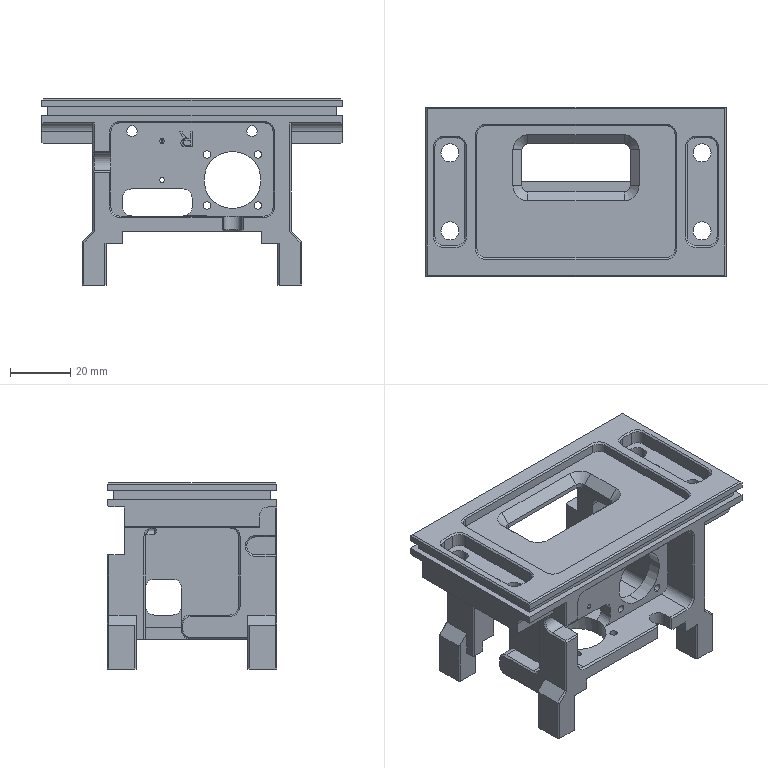NC program | Mastercam | posted with a generic post | part box 100 x 56.5 x 62 mm
Lines 29583 to 31427 of 47040, first 1520 of 1845 lines:
N8650 T16 M6
N8660 G0 G90 G17 G54 X59.62 Y2.263 A0. S5000 M3
N8670 G43 H16 Z20. M8
N8680 Z1.
N8690 G1 Z-28.5 F600.
N8700 X58.489 Y1.131 F1000.
N8710 G3 X58.02 Y0. I1.131 J-1.131
N8720 G1 Y-31.
N8730 G2 X50. Y-39.02 I-8.02 J0.
N8740 G1 X-50.
N8750 G2 X-58.02 Y-31. I0. J8.02
N8760 G1 Y31.
N8770 G2 X-50. Y39.02 I8.02 J0.
N8780 G1 X50.
N8790 G2 X58.02 Y31. I0. J-8.02
N8800 G1 Y0.
N8810 Y-.5
N8820 G3 X58.489 Y-1.631 I1.6 J0.
N8830 G1 X59.62 Y-2.763
N8840 G0 Z20.
N8850 Y2.263
N8860 Z1.
N8870 G1 Z-28.5 F600.
N8880 X58.489 Y1.131 F1000.
N8890 G3 X58.02 Y0. I1.131 J-1.131
N8900 G1 Y-31.
N8910 G2 X50. Y-39.02 I-8.02 J0.
N8920 G1 X-50.
N8930 G2 X-58.02 Y-31. I0. J8.02
N8940 G1 Y31.
N8950 G2 X-50. Y39.02 I8.02 J0.
N8960 G1 X50.
N8970 G2 X58.02 Y31. I0. J-8.02
N8980 G1 Y0.
N8990 Y-.5
N9000 G3 X58.489 Y-1.631 I1.6 J0.
N9010 G1 X59.62 Y-2.763
N9020 Y2.263
N9030 Z-57. F600.
N9040 X58.489 Y1.131 F1000.
N9050 G3 X58.02 Y0. I1.131 J-1.131
N9060 G1 Y-31.
N9070 G2 X50. Y-39.02 I-8.02 J0.
N9080 G1 X-50.
N9090 G2 X-58.02 Y-31. I0. J8.02
N9100 G1 Y31.
N9110 G2 X-50. Y39.02 I8.02 J0.
N9120 G1 X50.
N9130 G2 X58.02 Y31. I0. J-8.02
N9140 G1 Y0.
N9150 Y-.5
N9160 G3 X58.489 Y-1.631 I1.6 J0.
N9170 G1 X59.62 Y-2.763
N9180 G0 Z20.
N9190 Y2.263
N9200 Z-27.5
N9210 G1 Z-57. F600.
N9220 X58.489 Y1.131 F1000.
N9230 G3 X58.02 Y0. I1.131 J-1.131
N9240 G1 Y-31.
N9250 G2 X50. Y-39.02 I-8.02 J0.
N9260 G1 X-50.
N9270 G2 X-58.02 Y-31. I0. J8.02
N9280 G1 Y31.
N9290 G2 X-50. Y39.02 I8.02 J0.
N9300 G1 X50.
N9310 G2 X58.02 Y31. I0. J-8.02
N9320 G1 Y0.
N9330 Y-.5
N9340 G3 X58.489 Y-1.631 I1.6 J0.
N9350 G1 X59.62 Y-2.763
N9360 G0 Z20.
N9370 M5
N9380 G91 G28 Z0. M9
N9390 A0.
N9400 M01
N9410 T6 M6
N9420 G0 G90 G17 G54 X16.314 Y-19.3 A0. S6500 M3
N9430 G43 H6 Z20. M8
N9440 Z1.
N9450 G1 Z-.496 F600.
N9460 X16.738 Y-19.724 F3000.
N9470 G3 X17.162 Y-19.9 I.424 J.424
N9480 G1 X23.9
N9490 Y-13.87
N9500 G3 X23.724 Y-13.445 I-.6 J0.
N9510 G1 X23.3 Y-13.021
N9520 X16.314 Y-19.3
N9530 Z-.992 F600.
N9540 X16.738 Y-19.724 F3000.
N9550 G3 X17.162 Y-19.9 I.424 J.424
N9560 G1 X23.9
N9570 Y-13.87
N9580 G3 X23.724 Y-13.445 I-.6 J0.
N9590 G1 X23.3 Y-13.021
N9600 X16.314 Y-19.3
N9610 Z-1.488 F600.
N9620 X16.738 Y-19.724 F3000.
N9630 G3 X17.162 Y-19.9 I.424 J.424
N9640 G1 X23.9
N9650 Y-13.87
N9660 G3 X23.724 Y-13.445 I-.6 J0.
N9670 G1 X23.3 Y-13.021
N9680 X16.314 Y-19.3
N9690 Z-1.983 F600.
N9700 X16.738 Y-19.724 F3000.
N9710 G3 X17.162 Y-19.9 I.424 J.424
N9720 G1 X23.9
N9730 Y-13.87
N9740 G3 X23.724 Y-13.445 I-.6 J0.
N9750 G1 X23.3 Y-13.021
N9760 X16.314 Y-19.3
N9770 Z-2.479 F600.
N9780 X16.738 Y-19.724 F3000.
N9790 G3 X17.162 Y-19.9 I.424 J.424
N9800 G1 X23.9
N9810 Y-13.87
N9820 G3 X23.724 Y-13.445 I-.6 J0.
N9830 G1 X23.3 Y-13.021
N9840 X16.314 Y-19.3
N9850 Z-2.975 F600.
N9860 X16.738 Y-19.724 F3000.
N9870 G3 X17.162 Y-19.9 I.424 J.424
N9880 G1 X23.9
N9890 Y-13.87
N9900 G3 X23.724 Y-13.445 I-.6 J0.
N9910 G1 X23.3 Y-13.021
N9920 X16.314 Y-19.3
N9930 Z-3.471 F600.
N9940 X16.738 Y-19.724 F3000.
N9950 G3 X17.162 Y-19.9 I.424 J.424
N9960 G1 X23.9
N9970 Y-13.87
N9980 G3 X23.724 Y-13.445 I-.6 J0.
N9990 G1 X23.3 Y-13.021
N100 X16.314 Y-19.3
N110 Z-3.967 F600.
N120 X16.738 Y-19.724 F3000.
N130 G3 X17.162 Y-19.9 I.424 J.424
N140 G1 X23.9
N150 Y-13.87
N160 G3 X23.724 Y-13.445 I-.6 J0.
N170 G1 X23.3 Y-13.021
N180 X16.314 Y-19.3
N190 Z-4.463 F600.
N200 X16.738 Y-19.724 F3000.
N210 G3 X17.162 Y-19.9 I.424 J.424
N220 G1 X23.9
N230 Y-13.87
N240 G3 X23.724 Y-13.445 I-.6 J0.
N250 G1 X23.3 Y-13.021
N260 X16.314 Y-19.3
N270 Z-4.958 F600.
N280 X16.738 Y-19.724 F3000.
N290 G3 X17.162 Y-19.9 I.424 J.424
N300 G1 X23.9
N310 Y-13.87
N320 G3 X23.724 Y-13.445 I-.6 J0.
N330 G1 X23.3 Y-13.021
N340 X16.314 Y-19.3
N350 Z-5.454 F600.
N360 X16.738 Y-19.724 F3000.
N370 G3 X17.162 Y-19.9 I.424 J.424
N380 G1 X23.9
N390 Y-13.87
N400 G3 X23.724 Y-13.445 I-.6 J0.
N410 G1 X23.3 Y-13.021
N420 X16.314 Y-19.3
N430 Z-5.95 F600.
N440 X16.738 Y-19.724 F3000.
N450 G3 X17.162 Y-19.9 I.424 J.424
N460 G1 X23.9
N470 Y-13.87
N480 G3 X23.724 Y-13.445 I-.6 J0.
N490 G1 X23.3 Y-13.021
N500 X16.314 Y-19.3
N510 Z-6.446 F600.
N520 X16.738 Y-19.724 F3000.
N530 G3 X17.162 Y-19.9 I.424 J.424
N540 G1 X23.9
N550 Y-13.87
N560 G3 X23.724 Y-13.445 I-.6 J0.
N570 G1 X23.3 Y-13.021
N580 X16.314 Y-19.3
N590 Z-6.942 F600.
N600 X16.738 Y-19.724 F3000.
N610 G3 X17.162 Y-19.9 I.424 J.424
N620 G1 X23.9
N630 Y-13.87
N640 G3 X23.724 Y-13.445 I-.6 J0.
N650 G1 X23.3 Y-13.021
N660 X16.314 Y-19.3
N670 Z-7.438 F600.
N680 X16.738 Y-19.724 F3000.
N690 G3 X17.162 Y-19.9 I.424 J.424
N700 G1 X23.9
N710 Y-13.87
N720 G3 X23.724 Y-13.445 I-.6 J0.
N730 G1 X23.3 Y-13.021
N740 X16.314 Y-19.3
N750 Z-7.933 F600.
N760 X16.738 Y-19.724 F3000.
N770 G3 X17.162 Y-19.9 I.424 J.424
N780 G1 X23.9
N790 Y-13.87
N800 G3 X23.724 Y-13.445 I-.6 J0.
N810 G1 X23.3 Y-13.021
N820 X16.314 Y-19.3
N830 Z-8.429 F600.
N840 X16.738 Y-19.724 F3000.
N850 G3 X17.162 Y-19.9 I.424 J.424
N860 G1 X23.9
N870 Y-13.87
N880 G3 X23.724 Y-13.445 I-.6 J0.
N890 G1 X23.3 Y-13.021
N900 X16.314 Y-19.3
N910 Z-8.925 F600.
N920 X16.738 Y-19.724 F3000.
N930 G3 X17.162 Y-19.9 I.424 J.424
N940 G1 X23.9
N950 Y-13.87
N960 G3 X23.724 Y-13.445 I-.6 J0.
N970 G1 X23.3 Y-13.021
N980 X16.314 Y-19.3
N990 Z-9.421 F600.
N1000 X16.738 Y-19.724 F3000.
N1010 G3 X17.162 Y-19.9 I.424 J.424
N1020 G1 X23.9
N1030 Y-13.87
N1040 G3 X23.724 Y-13.445 I-.6 J0.
N1050 G1 X23.3 Y-13.021
N1060 X16.314 Y-19.3
N1070 Z-9.917 F600.
N1080 X16.738 Y-19.724 F3000.
N1090 G3 X17.162 Y-19.9 I.424 J.424
N1100 G1 X23.9
N1110 Y-13.87
N1120 G3 X23.724 Y-13.445 I-.6 J0.
N1130 G1 X23.3 Y-13.021
N1140 X16.314 Y-19.3
N1150 Z-10.412 F600.
N1160 X16.738 Y-19.724 F3000.
N1170 G3 X17.162 Y-19.9 I.424 J.424
N1180 G1 X23.9
N1190 Y-13.87
N1200 G3 X23.724 Y-13.445 I-.6 J0.
N1210 G1 X23.3 Y-13.021
N1220 X16.314 Y-19.3
N1230 Z-10.908 F600.
N1240 X16.738 Y-19.724 F3000.
N1250 G3 X17.162 Y-19.9 I.424 J.424
N1260 G1 X23.9
N1270 Y-13.87
N1280 G3 X23.724 Y-13.445 I-.6 J0.
N1290 G1 X23.3 Y-13.021
N1300 X16.314 Y-19.3
N1310 Z-11.404 F600.
N1320 X16.738 Y-19.724 F3000.
N1330 G3 X17.162 Y-19.9 I.424 J.424
N1340 G1 X23.9
N1350 Y-13.87
N1360 G3 X23.724 Y-13.445 I-.6 J0.
N1370 G1 X23.3 Y-13.021
N1380 X16.314 Y-19.3
N1390 Z-11.9 F600.
N1400 X16.738 Y-19.724 F3000.
N1410 G3 X17.162 Y-19.9 I.424 J.424
N1420 G1 X23.9
N1430 Y-13.87
N1440 G3 X23.724 Y-13.445 I-.6 J0.
N1450 G1 X23.3 Y-13.021
N1460 G0 Z20.
N1470 X-23.3 Y-13.011
N1480 Z1.
N1490 G1 Z-.496 F600.
N1500 X-23.724 Y-13.435 F3000.
N1510 G3 X-23.9 Y-13.859 I.424 J-.424
N1520 G1 Y-19.9
N1530 X-17.162
N1540 G3 X-16.738 Y-19.724 I0. J.6
N1550 G1 X-16.314 Y-19.3
N1560 X-23.3 Y-13.011
N1570 Z-.992 F600.
N1580 X-23.724 Y-13.435 F3000.
N1590 G3 X-23.9 Y-13.859 I.424 J-.424
N1600 G1 Y-19.9
N1610 X-17.162
N1620 G3 X-16.738 Y-19.724 I0. J.6
N1630 G1 X-16.314 Y-19.3
N1640 X-23.3 Y-13.011
N1650 Z-1.488 F600.
N1660 X-23.724 Y-13.435 F3000.
N1670 G3 X-23.9 Y-13.859 I.424 J-.424
N1680 G1 Y-19.9
N1690 X-17.162
N1700 G3 X-16.738 Y-19.724 I0. J.6
N1710 G1 X-16.314 Y-19.3
N1720 X-23.3 Y-13.011
N1730 Z-1.983 F600.
N1740 X-23.724 Y-13.435 F3000.
N1750 G3 X-23.9 Y-13.859 I.424 J-.424
N1760 G1 Y-19.9
N1770 X-17.162
N1780 G3 X-16.738 Y-19.724 I0. J.6
N1790 G1 X-16.314 Y-19.3
N1800 X-23.3 Y-13.011
N1810 Z-2.479 F600.
N1820 X-23.724 Y-13.435 F3000.
N1830 G3 X-23.9 Y-13.859 I.424 J-.424
N1840 G1 Y-19.9
N1850 X-17.162
N1860 G3 X-16.738 Y-19.724 I0. J.6
N1870 G1 X-16.314 Y-19.3
N1880 X-23.3 Y-13.011
N1890 Z-2.975 F600.
N1900 X-23.724 Y-13.435 F3000.
N1910 G3 X-23.9 Y-13.859 I.424 J-.424
N1920 G1 Y-19.9
N1930 X-17.162
N1940 G3 X-16.738 Y-19.724 I0. J.6
N1950 G1 X-16.314 Y-19.3
N1960 X-23.3 Y-13.011
N1970 Z-3.471 F600.
N1980 X-23.724 Y-13.435 F3000.
N1990 G3 X-23.9 Y-13.859 I.424 J-.424
N2000 G1 Y-19.9
N2010 X-17.162
N2020 G3 X-16.738 Y-19.724 I0. J.6
N2030 G1 X-16.314 Y-19.3
N2040 X-23.3 Y-13.011
N2050 Z-3.967 F600.
N2060 X-23.724 Y-13.435 F3000.
N2070 G3 X-23.9 Y-13.859 I.424 J-.424
N2080 G1 Y-19.9
N2090 X-17.162
N2100 G3 X-16.738 Y-19.724 I0. J.6
N2110 G1 X-16.314 Y-19.3
N2120 X-23.3 Y-13.011
N2130 Z-4.463 F600.
N2140 X-23.724 Y-13.435 F3000.
N2150 G3 X-23.9 Y-13.859 I.424 J-.424
N2160 G1 Y-19.9
N2170 X-17.162
N2180 G3 X-16.738 Y-19.724 I0. J.6
N2190 G1 X-16.314 Y-19.3
N2200 X-23.3 Y-13.011
N2210 Z-4.958 F600.
N2220 X-23.724 Y-13.435 F3000.
N2230 G3 X-23.9 Y-13.859 I.424 J-.424
N2240 G1 Y-19.9
N2250 X-17.162
N2260 G3 X-16.738 Y-19.724 I0. J.6
N2270 G1 X-16.314 Y-19.3
N2280 X-23.3 Y-13.011
N2290 Z-5.454 F600.
N2300 X-23.724 Y-13.435 F3000.
N2310 G3 X-23.9 Y-13.859 I.424 J-.424
N2320 G1 Y-19.9
N2330 X-17.162
N2340 G3 X-16.738 Y-19.724 I0. J.6
N2350 G1 X-16.314 Y-19.3
N2360 X-23.3 Y-13.011
N2370 Z-5.95 F600.
N2380 X-23.724 Y-13.435 F3000.
N2390 G3 X-23.9 Y-13.859 I.424 J-.424
N2400 G1 Y-19.9
N2410 X-17.162
N2420 G3 X-16.738 Y-19.724 I0. J.6
N2430 G1 X-16.314 Y-19.3
N2440 X-23.3 Y-13.011
N2450 Z-6.446 F600.
N2460 X-23.724 Y-13.435 F3000.
N2470 G3 X-23.9 Y-13.859 I.424 J-.424
N2480 G1 Y-19.9
N2490 X-17.162
N2500 G3 X-16.738 Y-19.724 I0. J.6
N2510 G1 X-16.314 Y-19.3
N2520 X-23.3 Y-13.011
N2530 Z-6.942 F600.
N2540 X-23.724 Y-13.435 F3000.
N2550 G3 X-23.9 Y-13.859 I.424 J-.424
N2560 G1 Y-19.9
N2570 X-17.162
N2580 G3 X-16.738 Y-19.724 I0. J.6
N2590 G1 X-16.314 Y-19.3
N2600 X-23.3 Y-13.011
N2610 Z-7.438 F600.
N2620 X-23.724 Y-13.435 F3000.
N2630 G3 X-23.9 Y-13.859 I.424 J-.424
N2640 G1 Y-19.9
N2650 X-17.162
N2660 G3 X-16.738 Y-19.724 I0. J.6
N2670 G1 X-16.314 Y-19.3
N2680 X-23.3 Y-13.011
N2690 Z-7.933 F600.
N2700 X-23.724 Y-13.435 F3000.
N2710 G3 X-23.9 Y-13.859 I.424 J-.424
N2720 G1 Y-19.9
N2730 X-17.162
N2740 G3 X-16.738 Y-19.724 I0. J.6
N2750 G1 X-16.314 Y-19.3
N2760 X-23.3 Y-13.011
N2770 Z-8.429 F600.
N2780 X-23.724 Y-13.435 F3000.
N2790 G3 X-23.9 Y-13.859 I.424 J-.424
N2800 G1 Y-19.9
N2810 X-17.162
N2820 G3 X-16.738 Y-19.724 I0. J.6
N2830 G1 X-16.314 Y-19.3
N2840 X-23.3 Y-13.011
N2850 Z-8.925 F600.
N2860 X-23.724 Y-13.435 F3000.
N2870 G3 X-23.9 Y-13.859 I.424 J-.424
N2880 G1 Y-19.9
N2890 X-17.162
N2900 G3 X-16.738 Y-19.724 I0. J.6
N2910 G1 X-16.314 Y-19.3
N2920 X-23.3 Y-13.011
N2930 Z-9.421 F600.
N2940 X-23.724 Y-13.435 F3000.
N2950 G3 X-23.9 Y-13.859 I.424 J-.424
N2960 G1 Y-19.9
N2970 X-17.162
N2980 G3 X-16.738 Y-19.724 I0. J.6
N2990 G1 X-16.314 Y-19.3
N3000 X-23.3 Y-13.011
N3010 Z-9.917 F600.
N3020 X-23.724 Y-13.435 F3000.
N3030 G3 X-23.9 Y-13.859 I.424 J-.424
N3040 G1 Y-19.9
N3050 X-17.162
N3060 G3 X-16.738 Y-19.724 I0. J.6
N3070 G1 X-16.314 Y-19.3
N3080 X-23.3 Y-13.011
N3090 Z-10.412 F600.
N3100 X-23.724 Y-13.435 F3000.
N3110 G3 X-23.9 Y-13.859 I.424 J-.424
N3120 G1 Y-19.9
N3130 X-17.162
N3140 G3 X-16.738 Y-19.724 I0. J.6
N3150 G1 X-16.314 Y-19.3
N3160 X-23.3 Y-13.011
N3170 Z-10.908 F600.
N3180 X-23.724 Y-13.435 F3000.
N3190 G3 X-23.9 Y-13.859 I.424 J-.424
N3200 G1 Y-19.9
N3210 X-17.162
N3220 G3 X-16.738 Y-19.724 I0. J.6
N3230 G1 X-16.314 Y-19.3
N3240 X-23.3 Y-13.011
N3250 Z-11.404 F600.
N3260 X-23.724 Y-13.435 F3000.
N3270 G3 X-23.9 Y-13.859 I.424 J-.424
N3280 G1 Y-19.9
N3290 X-17.162
N3300 G3 X-16.738 Y-19.724 I0. J.6
N3310 G1 X-16.314 Y-19.3
N3320 X-23.3 Y-13.011
N3330 Z-11.9 F600.
N3340 X-23.724 Y-13.435 F3000.
N3350 G3 X-23.9 Y-13.859 I.424 J-.424
N3360 G1 Y-19.9
N3370 X-17.162
N3380 G3 X-16.738 Y-19.724 I0. J.6
N3390 G1 X-16.314 Y-19.3
N3400 G0 Z20.
N3410 X-16.603 Y4.3
N3420 Z1.
N3430 G1 Z-.496 F600.
N3440 X-17.027 Y4.724 F3000.
N3450 G3 X-17.451 Y4.9 I-.424 J-.424
N3460 G1 X-23.9
N3470 Y-1.142
N3480 G3 X-23.724 Y-1.567 I.6 J0.
N3490 G1 X-23.3 Y-1.991
N3500 X-16.603 Y4.3
N3510 Z-.992 F600.
N3520 X-17.027 Y4.724 F3000.
N3530 G3 X-17.451 Y4.9 I-.424 J-.424
N3540 G1 X-23.9
N3550 Y-1.142
N3560 G3 X-23.724 Y-1.567 I.6 J0.
N3570 G1 X-23.3 Y-1.991
N3580 X-16.603 Y4.3
N3590 Z-1.488 F600.
N3600 X-17.027 Y4.724 F3000.
N3610 G3 X-17.451 Y4.9 I-.424 J-.424
N3620 G1 X-23.9
N3630 Y-1.142
N3640 G3 X-23.724 Y-1.567 I.6 J0.
N3650 G1 X-23.3 Y-1.991
N3660 X-16.603 Y4.3
N3670 Z-1.983 F600.
N3680 X-17.027 Y4.724 F3000.
N3690 G3 X-17.451 Y4.9 I-.424 J-.424
N3700 G1 X-23.9
N3710 Y-1.142
N3720 G3 X-23.724 Y-1.567 I.6 J0.
N3730 G1 X-23.3 Y-1.991
N3740 X-16.603 Y4.3
N3750 Z-2.479 F600.
N3760 X-17.027 Y4.724 F3000.
N3770 G3 X-17.451 Y4.9 I-.424 J-.424
N3780 G1 X-23.9
N3790 Y-1.142
N3800 G3 X-23.724 Y-1.567 I.6 J0.
N3810 G1 X-23.3 Y-1.991
N3820 X-16.603 Y4.3
N3830 Z-2.975 F600.
N3840 X-17.027 Y4.724 F3000.
N3850 G3 X-17.451 Y4.9 I-.424 J-.424
N3860 G1 X-23.9
N3870 Y-1.142
N3880 G3 X-23.724 Y-1.567 I.6 J0.
N3890 G1 X-23.3 Y-1.991
N3900 X-16.603 Y4.3
N3910 Z-3.471 F600.
N3920 X-17.027 Y4.724 F3000.
N3930 G3 X-17.451 Y4.9 I-.424 J-.424
N3940 G1 X-23.9
N3950 Y-1.142
N3960 G3 X-23.724 Y-1.567 I.6 J0.
N3970 G1 X-23.3 Y-1.991
N3980 X-16.603 Y4.3
N3990 Z-3.967 F600.
N4000 X-17.027 Y4.724 F3000.
N4010 G3 X-17.451 Y4.9 I-.424 J-.424
N4020 G1 X-23.9
N4030 Y-1.142
N4040 G3 X-23.724 Y-1.567 I.6 J0.
N4050 G1 X-23.3 Y-1.991
N4060 X-16.603 Y4.3
N4070 Z-4.463 F600.
N4080 X-17.027 Y4.724 F3000.
N4090 G3 X-17.451 Y4.9 I-.424 J-.424
N4100 G1 X-23.9
N4110 Y-1.142
N4120 G3 X-23.724 Y-1.567 I.6 J0.
N4130 G1 X-23.3 Y-1.991
N4140 X-16.603 Y4.3
N4150 Z-4.958 F600.
N4160 X-17.027 Y4.724 F3000.
N4170 G3 X-17.451 Y4.9 I-.424 J-.424
N4180 G1 X-23.9
N4190 Y-1.142
N4200 G3 X-23.724 Y-1.567 I.6 J0.
N4210 G1 X-23.3 Y-1.991
N4220 X-16.603 Y4.3
N4230 Z-5.454 F600.
N4240 X-17.027 Y4.724 F3000.
N4250 G3 X-17.451 Y4.9 I-.424 J-.424
N4260 G1 X-23.9
N4270 Y-1.142
N4280 G3 X-23.724 Y-1.567 I.6 J0.
N4290 G1 X-23.3 Y-1.991
N4300 X-16.603 Y4.3
N4310 Z-5.95 F600.
N4320 X-17.027 Y4.724 F3000.
N4330 G3 X-17.451 Y4.9 I-.424 J-.424
N4340 G1 X-23.9
N4350 Y-1.142
N4360 G3 X-23.724 Y-1.567 I.6 J0.
N4370 G1 X-23.3 Y-1.991
N4380 X-16.603 Y4.3
N4390 Z-6.446 F600.
N4400 X-17.027 Y4.724 F3000.
N4410 G3 X-17.451 Y4.9 I-.424 J-.424
N4420 G1 X-23.9
N4430 Y-1.142
N4440 G3 X-23.724 Y-1.567 I.6 J0.
N4450 G1 X-23.3 Y-1.991
N4460 X-16.603 Y4.3
N4470 Z-6.942 F600.
N4480 X-17.027 Y4.724 F3000.
N4490 G3 X-17.451 Y4.9 I-.424 J-.424
N4500 G1 X-23.9
N4510 Y-1.142
N4520 G3 X-23.724 Y-1.567 I.6 J0.
N4530 G1 X-23.3 Y-1.991
N4540 X-16.603 Y4.3
N4550 Z-7.438 F600.
N4560 X-17.027 Y4.724 F3000.
N4570 G3 X-17.451 Y4.9 I-.424 J-.424
N4580 G1 X-23.9
N4590 Y-1.142
N4600 G3 X-23.724 Y-1.567 I.6 J0.
N4610 G1 X-23.3 Y-1.991
N4620 X-16.603 Y4.3
N4630 Z-7.933 F600.
N4640 X-17.027 Y4.724 F3000.
N4650 G3 X-17.451 Y4.9 I-.424 J-.424
N4660 G1 X-23.9
N4670 Y-1.142
N4680 G3 X-23.724 Y-1.567 I.6 J0.
N4690 G1 X-23.3 Y-1.991
N4700 X-16.603 Y4.3
N4710 Z-8.429 F600.
N4720 X-17.027 Y4.724 F3000.
N4730 G3 X-17.451 Y4.9 I-.424 J-.424
N4740 G1 X-23.9
N4750 Y-1.142
N4760 G3 X-23.724 Y-1.567 I.6 J0.
N4770 G1 X-23.3 Y-1.991
N4780 X-16.603 Y4.3
N4790 Z-8.925 F600.
N4800 X-17.027 Y4.724 F3000.
N4810 G3 X-17.451 Y4.9 I-.424 J-.424
N4820 G1 X-23.9
N4830 Y-1.142
N4840 G3 X-23.724 Y-1.567 I.6 J0.
N4850 G1 X-23.3 Y-1.991
N4860 X-16.603 Y4.3
N4870 Z-9.421 F600.
N4880 X-17.027 Y4.724 F3000.
N4890 G3 X-17.451 Y4.9 I-.424 J-.424
N4900 G1 X-23.9
N4910 Y-1.142
N4920 G3 X-23.724 Y-1.567 I.6 J0.
N4930 G1 X-23.3 Y-1.991
N4940 X-16.603 Y4.3
N4950 Z-9.917 F600.
N4960 X-17.027 Y4.724 F3000.
N4970 G3 X-17.451 Y4.9 I-.424 J-.424
N4980 G1 X-23.9
N4990 Y-1.142
N5000 G3 X-23.724 Y-1.567 I.6 J0.
N5010 G1 X-23.3 Y-1.991
N5020 X-16.603 Y4.3
N5030 Z-10.412 F600.
N5040 X-17.027 Y4.724 F3000.
N5050 G3 X-17.451 Y4.9 I-.424 J-.424
N5060 G1 X-23.9
N5070 Y-1.142
N5080 G3 X-23.724 Y-1.567 I.6 J0.
N5090 G1 X-23.3 Y-1.991
N5100 X-16.603 Y4.3
N5110 Z-10.908 F600.
N5120 X-17.027 Y4.724 F3000.
N5130 G3 X-17.451 Y4.9 I-.424 J-.424
N5140 G1 X-23.9
N5150 Y-1.142
N5160 G3 X-23.724 Y-1.567 I.6 J0.
N5170 G1 X-23.3 Y-1.991
N5180 X-16.603 Y4.3
N5190 Z-11.404 F600.
N5200 X-17.027 Y4.724 F3000.
N5210 G3 X-17.451 Y4.9 I-.424 J-.424
N5220 G1 X-23.9
N5230 Y-1.142
N5240 G3 X-23.724 Y-1.567 I.6 J0.
N5250 G1 X-23.3 Y-1.991
N5260 X-16.603 Y4.3
N5270 Z-11.9 F600.
N5280 X-17.027 Y4.724 F3000.
N5290 G3 X-17.451 Y4.9 I-.424 J-.424
N5300 G1 X-23.9
N5310 Y-1.142
N5320 G3 X-23.724 Y-1.567 I.6 J0.
N5330 G1 X-23.3 Y-1.991
N5340 G0 Z20.
N5350 X23.3
N5360 Z1.
N5370 G1 Z-.496 F600.
N5380 X23.724 Y-1.566 F3000.
N5390 G3 X23.9 Y-1.142 I-.424 J.424
N5400 G1 Y4.9
N5410 X20.346
N5420 G2 X20.271 Y4.899 I-.075 J3.099
N5430 G1 X17.439
N5440 G3 X17.015 Y4.724 I0. J-.6
N5450 G1 X16.591 Y4.299
N5460 X23.3 Y-1.991
N5470 Z-.992 F600.
N5480 X23.724 Y-1.566 F3000.
N5490 G3 X23.9 Y-1.142 I-.424 J.424
N5500 G1 Y4.9
N5510 X20.346
N5520 G2 X20.271 Y4.899 I-.075 J3.099
N5530 G1 X17.439
N5540 G3 X17.015 Y4.724 I0. J-.6
N5550 G1 X16.591 Y4.299
N5560 X23.3 Y-1.991
N5570 Z-1.488 F600.
N5580 X23.724 Y-1.566 F3000.
N5590 G3 X23.9 Y-1.142 I-.424 J.424
N5600 G1 Y4.9
N5610 X20.346
N5620 G2 X20.271 Y4.899 I-.075 J3.099
N5630 G1 X17.439
N5640 G3 X17.015 Y4.724 I0. J-.6
N5650 G1 X16.591 Y4.299
N5660 X23.3 Y-1.991
N5670 Z-1.983 F600.
N5680 X23.724 Y-1.566 F3000.
N5690 G3 X23.9 Y-1.142 I-.424 J.424
N5700 G1 Y4.9
N5710 X20.346
N5720 G2 X20.271 Y4.899 I-.075 J3.099
N5730 G1 X17.439
N5740 G3 X17.015 Y4.724 I0. J-.6
N5750 G1 X16.591 Y4.299
N5760 X23.3 Y-1.991
N5770 Z-2.479 F600.
N5780 X23.724 Y-1.566 F3000.
N5790 G3 X23.9 Y-1.142 I-.424 J.424
N5800 G1 Y4.9
N5810 X20.346
N5820 G2 X20.271 Y4.899 I-.075 J3.099
N5830 G1 X17.439
N5840 G3 X17.015 Y4.724 I0. J-.6
N5850 G1 X16.591 Y4.299
N5860 X23.3 Y-1.991
N5870 Z-2.975 F600.
N5880 X23.724 Y-1.566 F3000.
N5890 G3 X23.9 Y-1.142 I-.424 J.424
N5900 G1 Y4.9
N5910 X20.346
N5920 G2 X20.271 Y4.899 I-.075 J3.099
N5930 G1 X17.439
N5940 G3 X17.015 Y4.724 I0. J-.6
N5950 G1 X16.591 Y4.299
N5960 X23.3 Y-1.991
N5970 Z-3.471 F600.
N5980 X23.724 Y-1.566 F3000.
N5990 G3 X23.9 Y-1.142 I-.424 J.424
N6000 G1 Y4.9
N6010 X20.346
N6020 G2 X20.271 Y4.899 I-.075 J3.099
N6030 G1 X17.439
N6040 G3 X17.015 Y4.724 I0. J-.6
N6050 G1 X16.591 Y4.299
N6060 X23.3 Y-1.991
N6070 Z-3.967 F600.
N6080 X23.724 Y-1.566 F3000.
N6090 G3 X23.9 Y-1.142 I-.424 J.424
N6100 G1 Y4.9
N6110 X20.346
N6120 G2 X20.271 Y4.899 I-.075 J3.099
N6130 G1 X17.439
N6140 G3 X17.015 Y4.724 I0. J-.6
N6150 G1 X16.591 Y4.299
N6160 X23.3 Y-1.991
N6170 Z-4.463 F600.
N6180 X23.724 Y-1.566 F3000.
N6190 G3 X23.9 Y-1.142 I-.424 J.424
N6200 G1 Y4.9
N6210 X20.346
N6220 G2 X20.271 Y4.899 I-.075 J3.099
N6230 G1 X17.439
N6240 G3 X17.015 Y4.724 I0. J-.6
N6250 G1 X16.591 Y4.299
N6260 X23.3 Y-1.991
N6270 Z-4.958 F600.
N6280 X23.724 Y-1.566 F3000.
N6290 G3 X23.9 Y-1.142 I-.424 J.424
N6300 G1 Y4.9
N6310 X20.346
N6320 G2 X20.271 Y4.899 I-.075 J3.099
N6330 G1 X17.439
N6340 G3 X17.015 Y4.724 I0. J-.6
N6350 G1 X16.591 Y4.299
N6360 X23.3 Y-1.991
N6370 Z-5.454 F600.
N6380 X23.724 Y-1.566 F3000.
N6390 G3 X23.9 Y-1.142 I-.424 J.424
N6400 G1 Y4.9
N6410 X20.346
N6420 G2 X20.271 Y4.899 I-.075 J3.099
N6430 G1 X17.439
N6440 G3 X17.015 Y4.724 I0. J-.6
N6450 G1 X16.591 Y4.299
N6460 X23.3 Y-1.991
N6470 Z-5.95 F600.
N6480 X23.724 Y-1.566 F3000.
N6490 G3 X23.9 Y-1.142 I-.424 J.424
N6500 G1 Y4.9
N6510 X20.346
N6520 G2 X20.271 Y4.899 I-.075 J3.099
N6530 G1 X17.439
N6540 G3 X17.015 Y4.724 I0. J-.6
N6550 G1 X16.591 Y4.299
N6560 X23.3 Y-1.991
N6570 Z-6.446 F600.
N6580 X23.724 Y-1.566 F3000.
N6590 G3 X23.9 Y-1.142 I-.424 J.424
N6600 G1 Y4.9
N6610 X20.346
N6620 G2 X20.271 Y4.899 I-.075 J3.099
N6630 G1 X17.439
N6640 G3 X17.015 Y4.724 I0. J-.6
N6650 G1 X16.591 Y4.299
N6660 X23.3 Y-1.991
N6670 Z-6.942 F600.
N6680 X23.724 Y-1.566 F3000.
N6690 G3 X23.9 Y-1.142 I-.424 J.424
N6700 G1 Y4.9
N6710 X20.346
N6720 G2 X20.271 Y4.899 I-.075 J3.099
N6730 G1 X17.439
N6740 G3 X17.015 Y4.724 I0. J-.6
N6750 G1 X16.591 Y4.299
N6760 X23.3 Y-1.991
N6770 Z-7.438 F600.
N6780 X23.724 Y-1.566 F3000.
N6790 G3 X23.9 Y-1.142 I-.424 J.424
N6800 G1 Y4.9
N6810 X20.346
N6820 G2 X20.271 Y4.899 I-.075 J3.099
N6830 G1 X17.439
N6840 G3 X17.015 Y4.724 I0. J-.6
N6850 G1 X16.591 Y4.299
N6860 X23.3 Y-1.991
N6870 Z-7.933 F600.
N6880 X23.724 Y-1.566 F3000.
N6890 G3 X23.9 Y-1.142 I-.424 J.424
N6900 G1 Y4.9
N6910 X20.346
N6920 G2 X20.271 Y4.899 I-.075 J3.099
N6930 G1 X17.439
N6940 G3 X17.015 Y4.724 I0. J-.6
N6950 G1 X16.591 Y4.299
N6960 X23.3 Y-1.991
N6970 Z-8.429 F600.
N6980 X23.724 Y-1.566 F3000.
N6990 G3 X23.9 Y-1.142 I-.424 J.424
N7000 G1 Y4.9
N7010 X20.346
N7020 G2 X20.271 Y4.899 I-.075 J3.099
N7030 G1 X17.439
N7040 G3 X17.015 Y4.724 I0. J-.6
N7050 G1 X16.591 Y4.299
N7060 X23.3 Y-1.991
N7070 Z-8.925 F600.
N7080 X23.724 Y-1.566 F3000.
N7090 G3 X23.9 Y-1.142 I-.424 J.424
N7100 G1 Y4.9
N7110 X20.346
N7120 G2 X20.271 Y4.899 I-.075 J3.099
N7130 G1 X17.439
N7140 G3 X17.015 Y4.724 I0. J-.6
N7150 G1 X16.591 Y4.299
N7160 X23.3 Y-1.991
N7170 Z-9.421 F600.
N7180 X23.724 Y-1.566 F3000.
N7190 G3 X23.9 Y-1.142 I-.424 J.424
N7200 G1 Y4.9
N7210 X20.346
N7220 G2 X20.271 Y4.899 I-.075 J3.099
N7230 G1 X17.439
N7240 G3 X17.015 Y4.724 I0. J-.6
N7250 G1 X16.591 Y4.299
N7260 X23.3 Y-1.991
N7270 Z-9.917 F600.
N7280 X23.724 Y-1.566 F3000.
N7290 G3 X23.9 Y-1.142 I-.424 J.424
N7300 G1 Y4.9
N7310 X20.346
N7320 G2 X20.271 Y4.899 I-.075 J3.099
N7330 G1 X17.439
N7340 G3 X17.015 Y4.724 I0. J-.6
N7350 G1 X16.591 Y4.299
N7360 X23.3 Y-1.991
N7370 Z-10.412 F600.
N7380 X23.724 Y-1.566 F3000.
N7390 G3 X23.9 Y-1.142 I-.424 J.424
N7400 G1 Y4.9
N7410 X20.346
N7420 G2 X20.271 Y4.899 I-.075 J3.099
N7430 G1 X17.439
N7440 G3 X17.015 Y4.724 I0. J-.6
N7450 G1 X16.591 Y4.299
N7460 X23.3 Y-1.991
N7470 Z-10.908 F600.
N7480 X23.724 Y-1.566 F3000.
N7490 G3 X23.9 Y-1.142 I-.424 J.424
N7500 G1 Y4.9
N7510 X20.346
N7520 G2 X20.271 Y4.899 I-.075 J3.099
N7530 G1 X17.439
N7540 G3 X17.015 Y4.724 I0. J-.6
N7550 G1 X16.591 Y4.299
N7560 X23.3 Y-1.991
N7570 Z-11.404 F600.
N7580 X23.724 Y-1.566 F3000.
N7590 G3 X23.9 Y-1.142 I-.424 J.424
N7600 G1 Y4.9
N7610 X20.346
N7620 G2 X20.271 Y4.899 I-.075 J3.099
N7630 G1 X17.439
N7640 G3 X17.015 Y4.724 I0. J-.6
N7650 G1 X16.591 Y4.299
N7660 X23.3 Y-1.991
N7670 Z-11.9 F600.
N7680 X23.724 Y-1.566 F3000.
N7690 G3 X23.9 Y-1.142 I-.424 J.424
N7700 G1 Y4.9
N7710 X20.346
N7720 G2 X20.271 Y4.899 I-.075 J3.099
N7730 G1 X17.439
N7740 G3 X17.015 Y4.724 I0. J-.6
N7750 G1 X16.591 Y4.299
N7760 G0 Z20.
N7770 X-1.114 Y-6.921
N7780 Z-11.
N7790 G1 Z-11.775 F600.
N7800 G3 X-6.814 Y-12.621 Z-11.831 I0. J-5.7 F1000.
N7810 X-1.114 Y-18.321 Z-11.887 I5.7 J0.
N7820 X4.586 Y-12.621 Z-11.944 I0. J5.7
N7830 X-1.114 Y-6.921 Z-12. I-5.7 J0.
N7840 G1 X-12.079
N7850 Y-8.08
N7860 X12.079
N7870 Y-6.921
N7880 X0.
N7890 X-1.114
N7900 G2 X-1.476 Y-6.63 I0. J.371
N7910 G1 X-1.865 Y-4.868
N7920 G3 X-2.227 Y-4.577 I-.362 J-.08
N7930 G1 X-14.423 Y-4.576
N7940 X-14.424 Y-10.424
N7950 X14.423
N7960 X14.424 Y-4.577
N7970 X0.
N7980 X-2.227
N7990 G2 X-2.59 Y-4.285 I0. J.372
N8000 G1 X-2.979 Y-2.524
N8010 G3 X-3.341 Y-2.233 I-.362 J-.08
N8020 G1 X-16.767 Y-2.232
N8030 X-16.768 Y-12.768
N8040 X16.767
N8050 X16.768 Y-2.233
N8060 X0.
N8070 X-3.341
N8080 G2 X-3.704 Y-1.941 I0. J.372
N8090 G1 X-4.092 Y-.18
N8100 G3 X-4.455 Y.112 I-.363 J-.08
N8110 G1 X-19.111
N8120 X-19.112 Y-15.112
N8130 X19.111
N8140 X19.112 Y.111
N8150 X0.
N8160 X-4.455 Y.112
N8170 G2 X-4.817 Y.403 I0. J.371
N8180 G1 X-5.206 Y2.164
N8190 G3 X-5.569 Y2.456 I-.363 J-.08
N8200 G1 X-21.455
N8210 X-21.456 Y-17.456
N8220 X21.455
N8230 X21.456 Y2.456
N8240 X0.
N8250 X-5.569
N8260 G2 X-5.931 Y2.747 I0. J.371
N8270 G1 X-6.32 Y4.508
N8280 G3 X-6.682 Y4.8 I-.362 J-.08
N8290 G1 X-23.799
N8300 X-23.8 Y-19.798
N8310 X-23.799 Y-19.8
N8320 X23.799
N8330 X23.8 Y4.798
N8340 X23.799 Y4.8
N8350 X0.
N8360 X-6.682
N8370 G0 Z20.
N8380 X12.448 Y4.38
N8390 Z1.
N8400 G1 Z-6. F600.
N8410 X12.024 Y4.804 F1000.
N8420 G3 X11.6 Y4.98 I-.424 J-.424
N8430 G1 X2.926
N8440 X-23.98
N8450 Y-19.98
N8460 X23.98
N8470 Y4.98
N8480 X20.274
N8490 X11.6
N8500 X11.1
N8510 G3 X10.676 Y4.804 I0. J-.6
N8520 G1 X10.251 Y4.38
N8530 X12.448 Y4.4 F500.
N8540 X12.024 Y4.824
N8550 G3 X11.6 Y5. I-.424 J-.424
N8560 G1 X2.926
N8570 X-24.
N8580 Y-20.
N8590 X24.
N8600 Y5.
N8610 X20.274
N8620 X11.6
N8630 X11.1
N8640 G3 X10.676 Y4.824 I0. J-.6
N8650 G1 X10.251 Y4.4
N8660 X12.448 Y4.38 F1000.
N8670 Z-12. F600.
N8680 X12.024 Y4.804 F1000.
N8690 G3 X11.6 Y4.98 I-.424 J-.424
N8700 G1 X2.926
N8710 X-23.98
N8720 Y-19.98
N8730 X23.98
N8740 Y4.98
N8750 X20.274
N8760 X11.6
N8770 X11.1
N8780 G3 X10.676 Y4.804 I0. J-.6
N8790 G1 X10.251 Y4.38
N8800 X12.448 Y4.4 F500.
N8810 X12.024 Y4.824
N8820 G3 X11.6 Y5. I-.424 J-.424
N8830 G1 X2.926
N8840 X-24.
N8850 Y-20.
N8860 X24.
N8870 Y5.
N8880 X20.274
N8890 X11.6
N8900 X11.1
N8910 G3 X10.676 Y4.824 I0. J-.6
N8920 G1 X10.251 Y4.4
N8930 G0 Z20.
N8940 X-13.5 Y-1.1
N8950 Z-11.
N8960 G1 Z-12. F600.
N8970 X-14.251 Y-1.199 Z-12.021 F1500.
N8980 X-14.95 Y-1.489 Z-12.042
N8990 X-15.551 Y-1.949 Z-12.063
N9000 X-16.011 Y-2.55 Z-12.083
N9010 X-16.301 Y-3.249 Z-12.104
N9020 X-16.4 Y-4. Z-12.125
N9030 X-16.301 Y-4.751 Z-12.146
N9040 X-16.011 Y-5.45 Z-12.167
N9050 X-15.551 Y-6.051 Z-12.188
N9060 X-14.95 Y-6.511 Z-12.208
N9070 X-14.251 Y-6.801 Z-12.229
N9080 X-13.5 Y-6.9 Z-12.25
N9090 X-12.749 Y-6.801 Z-12.271
N9100 X-12.05 Y-6.511 Z-12.292
N9110 X-11.449 Y-6.051 Z-12.313
N9120 X-10.989 Y-5.45 Z-12.333
N9130 X-10.699 Y-4.751 Z-12.354
N9140 X-10.6 Y-4. Z-12.375
N9150 X-10.699 Y-3.249 Z-12.396
N9160 X-10.989 Y-2.55 Z-12.417
N9170 X-11.449 Y-1.949 Z-12.438
N9180 X-12.05 Y-1.489 Z-12.458
N9190 X-12.749 Y-1.199 Z-12.479
N9200 X-13.5 Y-1.1 Z-12.5
N9210 X-14.251 Y-1.199 Z-12.521
N9220 X-14.95 Y-1.489 Z-12.542
N9230 X-15.551 Y-1.949 Z-12.563
N9240 X-16.011 Y-2.55 Z-12.583
N9250 X-16.301 Y-3.249 Z-12.604
N9260 X-16.4 Y-4. Z-12.625
N9270 X-16.301 Y-4.751 Z-12.646
N9280 X-16.011 Y-5.45 Z-12.667
N9290 X-15.551 Y-6.051 Z-12.688
N9300 X-14.95 Y-6.511 Z-12.708
N9310 X-14.251 Y-6.801 Z-12.729
N9320 X-13.5 Y-6.9 Z-12.75
N9330 X-12.749 Y-6.801 Z-12.771
N9340 X-12.05 Y-6.511 Z-12.792
N9350 X-11.449 Y-6.051 Z-12.813
N9360 X-10.989 Y-5.45 Z-12.833
N9370 X-10.699 Y-4.751 Z-12.854
N9380 X-10.6 Y-4. Z-12.875
N9390 X-10.699 Y-3.249 Z-12.896
N9400 X-10.989 Y-2.55 Z-12.917
N9410 X-11.449 Y-1.949 Z-12.938
N9420 X-12.05 Y-1.489 Z-12.958
N9430 X-12.749 Y-1.199 Z-12.979
N9440 X-13.5 Y-1.1 Z-13.
N9450 X-14.251 Y-1.199 Z-13.021
N9460 X-14.95 Y-1.489 Z-13.042
N9470 X-15.551 Y-1.949 Z-13.063
N9480 X-16.011 Y-2.55 Z-13.083
N9490 X-16.301 Y-3.249 Z-13.104
N9500 X-16.4 Y-4. Z-13.125
N9510 X-16.301 Y-4.751 Z-13.146
N9520 X-16.011 Y-5.45 Z-13.167
N9530 X-15.551 Y-6.051 Z-13.188
N9540 X-14.95 Y-6.511 Z-13.208
N9550 X-14.251 Y-6.801 Z-13.229
N9560 X-13.5 Y-6.9 Z-13.25
N9570 X-12.749 Y-6.801 Z-13.271
N9580 X-12.05 Y-6.511 Z-13.292
N9590 X-11.449 Y-6.051 Z-13.313
N9600 X-10.989 Y-5.45 Z-13.333
N9610 X-10.699 Y-4.751 Z-13.354
N9620 X-10.6 Y-4. Z-13.375
N9630 X-10.699 Y-3.249 Z-13.396
N9640 X-10.989 Y-2.55 Z-13.417
N9650 X-11.449 Y-1.949 Z-13.438
N9660 X-12.05 Y-1.489 Z-13.458
N9670 X-12.749 Y-1.199 Z-13.479
N9680 X-13.5 Y-1.1 Z-13.5
N9690 X-14.251 Y-1.199 Z-13.521
N9700 X-14.95 Y-1.489 Z-13.542
N9710 X-15.551 Y-1.949 Z-13.563
N9720 X-16.011 Y-2.55 Z-13.583
N9730 X-16.301 Y-3.249 Z-13.604
N9740 X-16.4 Y-4. Z-13.625
N9750 X-16.301 Y-4.751 Z-13.646
N9760 X-16.011 Y-5.45 Z-13.667
N9770 X-15.551 Y-6.051 Z-13.688
N9780 X-14.95 Y-6.511 Z-13.708
N9790 X-14.251 Y-6.801 Z-13.729
N9800 X-13.5 Y-6.9 Z-13.75
N9810 X-12.749 Y-6.801 Z-13.771
N9820 X-12.05 Y-6.511 Z-13.792
N9830 X-11.449 Y-6.051 Z-13.813
N9840 X-10.989 Y-5.45 Z-13.833
N9850 X-10.699 Y-4.751 Z-13.854
N9860 X-10.6 Y-4. Z-13.875
N9870 X-10.699 Y-3.249 Z-13.896
N9880 X-10.989 Y-2.55 Z-13.917
N9890 X-11.449 Y-1.949 Z-13.938
N9900 X-12.05 Y-1.489 Z-13.958
N9910 X-12.749 Y-1.199 Z-13.979
N9920 X-13.5 Y-1.1 Z-14.
N9930 X-14.251 Y-1.199 Z-14.021
N9940 X-14.95 Y-1.489 Z-14.042
N9950 X-15.551 Y-1.949 Z-14.063
N9960 X-16.011 Y-2.55 Z-14.083
N9970 X-16.301 Y-3.249 Z-14.104
N9980 X-16.4 Y-4. Z-14.125
N9990 X-16.301 Y-4.751 Z-14.146
N100 X-16.011 Y-5.45 Z-14.167
N110 X-15.551 Y-6.051 Z-14.188
N120 X-14.95 Y-6.511 Z-14.208
N130 X-14.251 Y-6.801 Z-14.229
N140 X-13.5 Y-6.9 Z-14.25
N150 X-12.749 Y-6.801 Z-14.271
N160 X-12.05 Y-6.511 Z-14.292
N170 X-11.449 Y-6.051 Z-14.313
N180 X-10.989 Y-5.45 Z-14.333
N190 X-10.699 Y-4.751 Z-14.354
N200 X-10.6 Y-4. Z-14.375
N210 X-10.699 Y-3.249 Z-14.396
N220 X-10.989 Y-2.55 Z-14.417
N230 X-11.449 Y-1.949 Z-14.438
N240 X-12.05 Y-1.489 Z-14.458
N250 X-12.749 Y-1.199 Z-14.479
N260 X-13.5 Y-1.1 Z-14.5
N270 X-14.251 Y-1.199 Z-14.521
N280 X-14.95 Y-1.489 Z-14.542
N290 X-15.551 Y-1.949 Z-14.563
N300 X-16.011 Y-2.55 Z-14.583
N310 X-16.301 Y-3.249 Z-14.604
N320 X-16.4 Y-4. Z-14.625
N330 X-16.301 Y-4.751 Z-14.646
N340 X-16.011 Y-5.45 Z-14.667
N350 X-15.551 Y-6.051 Z-14.688
N360 X-14.95 Y-6.511 Z-14.708
N370 X-14.251 Y-6.801 Z-14.729
N380 X-13.5 Y-6.9 Z-14.75
N390 X-12.749 Y-6.801 Z-14.771
N400 X-12.05 Y-6.511 Z-14.792
N410 X-11.449 Y-6.051 Z-14.813
N420 X-10.989 Y-5.45 Z-14.833
N430 X-10.699 Y-4.751 Z-14.854
N440 X-10.6 Y-4. Z-14.875
N450 X-10.699 Y-3.249 Z-14.896
N460 X-10.989 Y-2.55 Z-14.917
N470 X-11.449 Y-1.949 Z-14.938
N480 X-12.05 Y-1.489 Z-14.958
N490 X-12.749 Y-1.199 Z-14.979
N500 X-13.5 Y-1.1 Z-15.
N510 X-14.251 Y-1.199 Z-15.021
N520 X-14.95 Y-1.489 Z-15.042
N530 X-15.551 Y-1.949 Z-15.063
N540 X-16.011 Y-2.55 Z-15.083
N550 X-16.301 Y-3.249 Z-15.104
N560 X-16.4 Y-4. Z-15.125
N570 X-16.301 Y-4.751 Z-15.146
N580 X-16.011 Y-5.45 Z-15.167
N590 X-15.551 Y-6.051 Z-15.188
N600 X-14.95 Y-6.511 Z-15.208
N610 X-14.251 Y-6.801 Z-15.229
N620 X-13.5 Y-6.9 Z-15.25
N630 X-12.749 Y-6.801 Z-15.271
N640 X-12.05 Y-6.511 Z-15.292
N650 X-11.449 Y-6.051 Z-15.313
N660 X-10.989 Y-5.45 Z-15.333
N670 X-10.699 Y-4.751 Z-15.354
N680 X-10.6 Y-4. Z-15.375
N690 X-10.699 Y-3.249 Z-15.396
N700 X-10.989 Y-2.55 Z-15.417
N710 X-11.449 Y-1.949 Z-15.438
N720 X-12.05 Y-1.489 Z-15.458
N730 X-12.749 Y-1.199 Z-15.479
N740 X-13.5 Y-1.1 Z-15.5
N750 X-14.251 Y-1.199 Z-15.521
N760 X-14.95 Y-1.489 Z-15.542
N770 X-15.551 Y-1.949 Z-15.563
N780 X-16.011 Y-2.55 Z-15.583
N790 X-16.301 Y-3.249 Z-15.604
N800 X-16.4 Y-4. Z-15.625
N810 X-16.301 Y-4.751 Z-15.646
N820 X-16.011 Y-5.45 Z-15.667
N830 X-15.551 Y-6.051 Z-15.688
N840 X-14.95 Y-6.511 Z-15.708
N850 X-14.251 Y-6.801 Z-15.729
N860 X-13.5 Y-6.9 Z-15.75
N870 X-12.749 Y-6.801 Z-15.771
N880 X-12.05 Y-6.511 Z-15.792
N890 X-11.449 Y-6.051 Z-15.813
N900 X-10.989 Y-5.45 Z-15.833
N910 X-10.699 Y-4.751 Z-15.854
N920 X-10.6 Y-4. Z-15.875
N930 X-10.699 Y-3.249 Z-15.896
N940 X-10.989 Y-2.55 Z-15.917
N950 X-11.449 Y-1.949 Z-15.938
N960 X-12.05 Y-1.489 Z-15.958
N970 X-12.749 Y-1.199 Z-15.979
N980 X-13.5 Y-1.1 Z-16.
N990 X-14.251 Y-1.199 Z-16.021
N1000 X-14.95 Y-1.489 Z-16.042
N1010 X-15.551 Y-1.949 Z-16.063
N1020 X-16.011 Y-2.55 Z-16.083
N1030 X-16.301 Y-3.249 Z-16.104
N1040 X-16.4 Y-4. Z-16.125
N1050 X-16.301 Y-4.751 Z-16.146
N1060 X-16.011 Y-5.45 Z-16.167
N1070 X-15.551 Y-6.051 Z-16.188
N1080 X-14.95 Y-6.511 Z-16.208
N1090 X-14.251 Y-6.801 Z-16.229
N1100 X-13.5 Y-6.9 Z-16.25
N1110 X-12.749 Y-6.801 Z-16.271
N1120 X-12.05 Y-6.511 Z-16.292
N1130 X-11.449 Y-6.051 Z-16.313
N1140 X-10.989 Y-5.45 Z-16.333
N1150 X-10.699 Y-4.751 Z-16.354
N1160 X-10.6 Y-4. Z-16.375
N1170 X-10.699 Y-3.249 Z-16.396
N1180 X-10.989 Y-2.55 Z-16.417
N1190 X-11.449 Y-1.949 Z-16.438
N1200 X-12.05 Y-1.489 Z-16.458
N1210 X-12.749 Y-1.199 Z-16.479
N1220 X-13.5 Y-1.1 Z-16.5
N1230 X-14.251 Y-1.199 Z-16.521
N1240 X-14.95 Y-1.489 Z-16.542
N1250 X-15.551 Y-1.949 Z-16.563
N1260 X-16.011 Y-2.55 Z-16.583
N1270 X-16.301 Y-3.249 Z-16.604
N1280 X-16.4 Y-4. Z-16.625
N1290 X-16.301 Y-4.751 Z-16.646
N1300 X-16.011 Y-5.45 Z-16.667
N1310 X-15.551 Y-6.051 Z-16.688
N1320 X-14.95 Y-6.511 Z-16.708
N1330 X-14.251 Y-6.801 Z-16.729
N1340 X-13.5 Y-6.9 Z-16.75
N1350 X-12.749 Y-6.801 Z-16.771
N1360 X-12.05 Y-6.511 Z-16.792
N1370 X-11.449 Y-6.051 Z-16.813
N1380 X-10.989 Y-5.45 Z-16.833
N1390 X-10.699 Y-4.751 Z-16.854
N1400 X-10.6 Y-4. Z-16.875
N1410 X-10.699 Y-3.249 Z-16.896
N1420 X-10.989 Y-2.55 Z-16.917
N1430 X-11.449 Y-1.949 Z-16.938
N1440 X-12.05 Y-1.489 Z-16.958
N1450 X-12.749 Y-1.199 Z-16.979
N1460 X-13.5 Y-1.1 Z-17.
N1470 G3 X-16.4 Y-4. I0. J-2.9
N1480 X-13.5 Y-6.9 I2.9 J0.
N1490 X-10.6 Y-4. I0. J2.9
N1500 X-13.5 Y-1.1 I-2.9 J0.
N1510 X-13.998 Y-1.143 I0. J-2.9
N1520 G0 Z20.
N1530 X-13.5 Y2.4
N1540 Z-11.
N1550 G1 Z-12. F600.
N1560 X-14.611 Y2.303 Z-12.014 F1500.
N1570 X-15.689 Y2.014 Z-12.028
N1580 X-16.7 Y1.543 Z-12.042
N1590 X-17.614 Y.903 Z-12.056
N1600 X-18.403 Y.114 Z-12.069
N1610 X-19.043 Y-.8 Z-12.083
N1620 X-19.514 Y-1.811 Z-12.097
N1630 X-19.803 Y-2.889 Z-12.111
N1640 X-19.9 Y-4. Z-12.125
N1650 X-19.803 Y-5.111 Z-12.139
N1660 X-19.514 Y-6.189 Z-12.153
N1670 X-19.043 Y-7.2 Z-12.167
N1680 X-18.403 Y-8.114 Z-12.181
N1690 X-17.614 Y-8.903 Z-12.194
N1700 X-16.7 Y-9.543 Z-12.208
N1710 X-15.689 Y-10.014 Z-12.222
N1720 X-14.611 Y-10.303 Z-12.236
N1730 X-13.5 Y-10.4 Z-12.25
N1740 X-12.389 Y-10.303 Z-12.264
N1750 X-11.311 Y-10.014 Z-12.278
N1760 X-10.3 Y-9.543 Z-12.292
N1770 X-9.386 Y-8.903 Z-12.306
N1780 X-8.597 Y-8.114 Z-12.319
N1790 X-7.957 Y-7.2 Z-12.333
N1800 X-7.486 Y-6.189 Z-12.347
N1810 X-7.197 Y-5.111 Z-12.361
N1820 X-7.1 Y-4. Z-12.375
N1830 X-7.197 Y-2.889 Z-12.389
N1840 X-7.486 Y-1.811 Z-12.403
N1850 X-7.957 Y-.8 Z-12.417
N1860 X-8.597 Y.114 Z-12.431
N1870 X-9.386 Y.903 Z-12.444
N1880 X-10.3 Y1.543 Z-12.458
N1890 X-11.311 Y2.014 Z-12.472
N1900 X-12.389 Y2.303 Z-12.486
N1910 X-13.5 Y2.4 Z-12.5
N1920 X-14.611 Y2.303 Z-12.514
N1930 X-15.689 Y2.014 Z-12.528
N1940 X-16.7 Y1.543 Z-12.542
N1950 X-17.614 Y.903 Z-12.556
N1960 X-18.403 Y.114 Z-12.569
N1970 X-19.043 Y-.8 Z-12.583
N1980 X-19.514 Y-1.811 Z-12.597
N1990 X-19.803 Y-2.889 Z-12.611
N2000 X-19.9 Y-4. Z-12.625
N2010 X-19.803 Y-5.111 Z-12.639
N2020 X-19.514 Y-6.189 Z-12.653
N2030 X-19.043 Y-7.2 Z-12.667
N2040 X-18.403 Y-8.114 Z-12.681
N2050 X-17.614 Y-8.903 Z-12.694
N2060 X-16.7 Y-9.543 Z-12.708
N2070 X-15.689 Y-10.014 Z-12.722
N2080 X-14.611 Y-10.303 Z-12.736
N2090 X-13.5 Y-10.4 Z-12.75
N2100 X-12.389 Y-10.303 Z-12.764
N2110 X-11.311 Y-10.014 Z-12.778
N2120 X-10.3 Y-9.543 Z-12.792
N2130 X-9.386 Y-8.903 Z-12.806
N2140 X-8.597 Y-8.114 Z-12.819
N2150 X-7.957 Y-7.2 Z-12.833
N2160 X-7.486 Y-6.189 Z-12.847
N2170 X-7.197 Y-5.111 Z-12.861
N2180 X-7.1 Y-4. Z-12.875
N2190 X-7.197 Y-2.889 Z-12.889
N2200 X-7.486 Y-1.811 Z-12.903
N2210 X-7.957 Y-.8 Z-12.917
N2220 X-8.597 Y.114 Z-12.931
N2230 X-9.386 Y.903 Z-12.944
N2240 X-10.3 Y1.543 Z-12.958
N2250 X-11.311 Y2.014 Z-12.972
N2260 X-12.389 Y2.303 Z-12.986
N2270 X-13.5 Y2.4 Z-13.
N2280 X-14.611 Y2.303 Z-13.014
N2290 X-15.689 Y2.014 Z-13.028
N2300 X-16.7 Y1.543 Z-13.042
N2310 X-17.614 Y.903 Z-13.056
N2320 X-18.403 Y.114 Z-13.069
N2330 X-19.043 Y-.8 Z-13.083
N2340 X-19.514 Y-1.811 Z-13.097
N2350 X-19.803 Y-2.889 Z-13.111
N2360 X-19.9 Y-4. Z-13.125
N2370 X-19.803 Y-5.111 Z-13.139
N2380 X-19.514 Y-6.189 Z-13.153
N2390 X-19.043 Y-7.2 Z-13.167
N2400 X-18.403 Y-8.114 Z-13.181
N2410 X-17.614 Y-8.903 Z-13.194
N2420 X-16.7 Y-9.543 Z-13.208
N2430 X-15.689 Y-10.014 Z-13.222
N2440 X-14.611 Y-10.303 Z-13.236
N2450 X-13.5 Y-10.4 Z-13.25
N2460 X-12.389 Y-10.303 Z-13.264
N2470 X-11.311 Y-10.014 Z-13.278
N2480 X-10.3 Y-9.543 Z-13.292
N2490 X-9.386 Y-8.903 Z-13.306
N2500 X-8.597 Y-8.114 Z-13.319
N2510 X-7.957 Y-7.2 Z-13.333
N2520 X-7.486 Y-6.189 Z-13.347
N2530 X-7.197 Y-5.111 Z-13.361
N2540 X-7.1 Y-4. Z-13.375
N2550 X-7.197 Y-2.889 Z-13.389
N2560 X-7.486 Y-1.811 Z-13.403
N2570 X-7.957 Y-.8 Z-13.417
N2580 X-8.597 Y.114 Z-13.431
N2590 X-9.386 Y.903 Z-13.444
N2600 X-10.3 Y1.543 Z-13.458
N2610 X-11.311 Y2.014 Z-13.472
N2620 X-12.389 Y2.303 Z-13.486
N2630 X-13.5 Y2.4 Z-13.5
N2640 X-14.611 Y2.303 Z-13.514
N2650 X-15.689 Y2.014 Z-13.528
N2660 X-16.7 Y1.543 Z-13.542
N2670 X-17.614 Y.903 Z-13.556
N2680 X-18.403 Y.114 Z-13.569
N2690 X-19.043 Y-.8 Z-13.583
N2700 X-19.514 Y-1.811 Z-13.597
N2710 X-19.803 Y-2.889 Z-13.611
N2720 X-19.9 Y-4. Z-13.625
N2730 X-19.803 Y-5.111 Z-13.639
N2740 X-19.514 Y-6.189 Z-13.653
N2750 X-19.043 Y-7.2 Z-13.667
N2760 X-18.403 Y-8.114 Z-13.681
N2770 X-17.614 Y-8.903 Z-13.694
N2780 X-16.7 Y-9.543 Z-13.708
N2790 X-15.689 Y-10.014 Z-13.722
N2800 X-14.611 Y-10.303 Z-13.736
N2810 X-13.5 Y-10.4 Z-13.75
N2820 X-12.389 Y-10.303 Z-13.764
N2830 X-11.311 Y-10.014 Z-13.778
N2840 X-10.3 Y-9.543 Z-13.792
N2850 X-9.386 Y-8.903 Z-13.806
N2860 X-8.597 Y-8.114 Z-13.819
N2870 X-7.957 Y-7.2 Z-13.833
N2880 X-7.486 Y-6.189 Z-13.847
N2890 X-7.197 Y-5.111 Z-13.861
N2900 X-7.1 Y-4. Z-13.875
N2910 X-7.197 Y-2.889 Z-13.889
N2920 X-7.486 Y-1.811 Z-13.903
N2930 X-7.957 Y-.8 Z-13.917
N2940 X-8.597 Y.114 Z-13.931
N2950 X-9.386 Y.903 Z-13.944
N2960 X-10.3 Y1.543 Z-13.958
N2970 X-11.311 Y2.014 Z-13.972
N2980 X-12.389 Y2.303 Z-13.986
N2990 X-13.5 Y2.4 Z-14.
N3000 X-14.611 Y2.303 Z-14.014
N3010 X-15.689 Y2.014 Z-14.028
N3020 X-16.7 Y1.543 Z-14.042
N3030 X-17.614 Y.903 Z-14.056
N3040 X-18.403 Y.114 Z-14.069
N3050 X-19.043 Y-.8 Z-14.083
N3060 X-19.514 Y-1.811 Z-14.097
N3070 X-19.803 Y-2.889 Z-14.111
N3080 X-19.9 Y-4. Z-14.125
N3090 X-19.803 Y-5.111 Z-14.139
N3100 X-19.514 Y-6.189 Z-14.153
N3110 X-19.043 Y-7.2 Z-14.167
N3120 X-18.403 Y-8.114 Z-14.181
N3130 X-17.614 Y-8.903 Z-14.194
N3140 X-16.7 Y-9.543 Z-14.208
N3150 X-15.689 Y-10.014 Z-14.222
N3160 X-14.611 Y-10.303 Z-14.236
N3170 X-13.5 Y-10.4 Z-14.25
N3180 X-12.389 Y-10.303 Z-14.264
N3190 X-11.311 Y-10.014 Z-14.278
N3200 X-10.3 Y-9.543 Z-14.292
N3210 X-9.386 Y-8.903 Z-14.306
N3220 X-8.597 Y-8.114 Z-14.319
N3230 X-7.957 Y-7.2 Z-14.333
N3240 X-7.486 Y-6.189 Z-14.347
N3250 X-7.197 Y-5.111 Z-14.361
N3260 X-7.1 Y-4. Z-14.375
N3270 X-7.197 Y-2.889 Z-14.389
N3280 X-7.486 Y-1.811 Z-14.403
N3290 X-7.957 Y-.8 Z-14.417
N3300 X-8.597 Y.114 Z-14.431
N3310 X-9.386 Y.903 Z-14.444
N3320 X-10.3 Y1.543 Z-14.458
N3330 X-11.311 Y2.014 Z-14.472
N3340 X-12.389 Y2.303 Z-14.486
N3350 X-13.5 Y2.4 Z-14.5
N3360 X-14.611 Y2.303 Z-14.514
N3370 X-15.689 Y2.014 Z-14.528
N3380 X-16.7 Y1.543 Z-14.542
N3390 X-17.614 Y.903 Z-14.556
N3400 X-18.403 Y.114 Z-14.569
N3410 X-19.043 Y-.8 Z-14.583
N3420 X-19.514 Y-1.811 Z-14.597
N3430 X-19.803 Y-2.889 Z-14.611
N3440 X-19.9 Y-4. Z-14.625
N3450 X-19.803 Y-5.111 Z-14.639
N3460 X-19.514 Y-6.189 Z-14.653
N3470 X-19.043 Y-7.2 Z-14.667
N3480 X-18.403 Y-8.114 Z-14.681
N3490 X-17.614 Y-8.903 Z-14.694
N3500 X-16.7 Y-9.543 Z-14.708
N3510 X-15.689 Y-10.014 Z-14.722
N3520 X-14.611 Y-10.303 Z-14.736
N3530 X-13.5 Y-10.4 Z-14.75
N3540 X-12.389 Y-10.303 Z-14.764
N3550 X-11.311 Y-10.014 Z-14.778
N3560 X-10.3 Y-9.543 Z-14.792
N3570 X-9.386 Y-8.903 Z-14.806
N3580 X-8.597 Y-8.114 Z-14.819
N3590 X-7.957 Y-7.2 Z-14.833
N3600 X-7.486 Y-6.189 Z-14.847
N3610 X-7.197 Y-5.111 Z-14.861
N3620 X-7.1 Y-4. Z-14.875
N3630 X-7.197 Y-2.889 Z-14.889
N3640 X-7.486 Y-1.811 Z-14.903
N3650 X-7.957 Y-.8 Z-14.917
N3660 X-8.597 Y.114 Z-14.931
N3670 X-9.386 Y.903 Z-14.944
N3680 X-10.3 Y1.543 Z-14.958
N3690 X-11.311 Y2.014 Z-14.972
N3700 X-12.389 Y2.303 Z-14.986
N3710 X-13.5 Y2.4 Z-15.
N3720 X-14.611 Y2.303 Z-15.014
N3730 X-15.689 Y2.014 Z-15.028
N3740 X-16.7 Y1.543 Z-15.042
N3750 X-17.614 Y.903 Z-15.056
N3760 X-18.403 Y.114 Z-15.069
N3770 X-19.043 Y-.8 Z-15.083
N3780 X-19.514 Y-1.811 Z-15.097
N3790 X-19.803 Y-2.889 Z-15.111
N3800 X-19.9 Y-4. Z-15.125
N3810 X-19.803 Y-5.111 Z-15.139
N3820 X-19.514 Y-6.189 Z-15.153
N3830 X-19.043 Y-7.2 Z-15.167
N3840 X-18.403 Y-8.114 Z-15.181
N3850 X-17.614 Y-8.903 Z-15.194
N3860 X-16.7 Y-9.543 Z-15.208
N3870 X-15.689 Y-10.014 Z-15.222
N3880 X-14.611 Y-10.303 Z-15.236
N3890 X-13.5 Y-10.4 Z-15.25
N3900 X-12.389 Y-10.303 Z-15.264
N3910 X-11.311 Y-10.014 Z-15.278
N3920 X-10.3 Y-9.543 Z-15.292
N3930 X-9.386 Y-8.903 Z-15.306
N3940 X-8.597 Y-8.114 Z-15.319
N3950 X-7.957 Y-7.2 Z-15.333
N3960 X-7.486 Y-6.189 Z-15.347
N3970 X-7.197 Y-5.111 Z-15.361
N3980 X-7.1 Y-4. Z-15.375
N3990 X-7.197 Y-2.889 Z-15.389
N4000 X-7.486 Y-1.811 Z-15.403
N4010 X-7.957 Y-.8 Z-15.417
N4020 X-8.597 Y.114 Z-15.431
N4030 X-9.386 Y.903 Z-15.444
N4040 X-10.3 Y1.543 Z-15.458